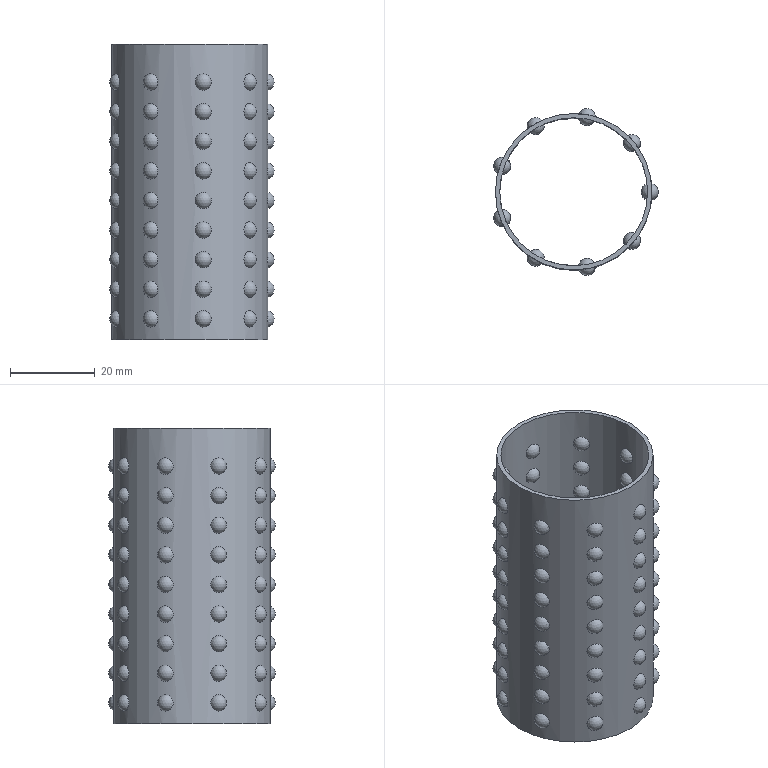Part | NX | features BREP 1 | 1 solid | 166 faces | box 38.914 x 39.453 x 70 mm | volume 9635 mm3 | sphere 162 | plane 2 | cylinder 2 | commonest cylinder face diameters 35 x1 37 x1